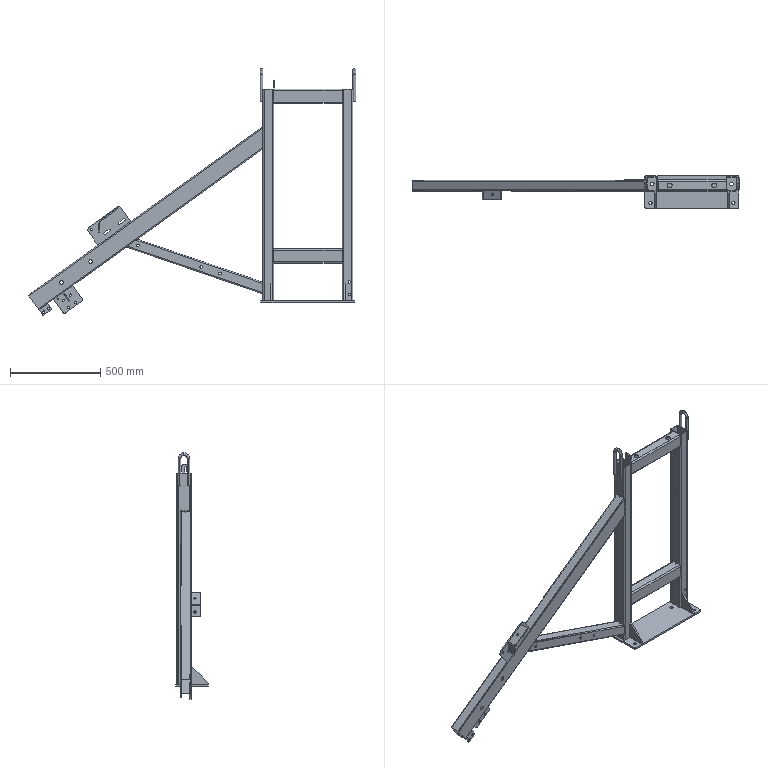Part | SolidWorks | features ICE 12, Cut 6, WeldCornerFeat 5, WeldMemberFeat 5, 3DProfileFeature 3, Gusset 3, HoleWzd 3, DeleteBody 2, MirrorSolid 2, MoveCopyBody 2, Extrusion 1, Fillet 1, FlatPattern 1, SM3dBend 1, SMBaseFlange 1, SheetMetal 1, Sweep 1, WeldmentFeature 1 | 17 solids | 340 faces | box 1815 x 180 x 1367 mm | volume 6438478 mm3 | plane 174 | cylinder 158 | torus 8 | commonest cylinder face diameters 14 x28 12 x25 8 x16 16 x16 20 x13 6 x9